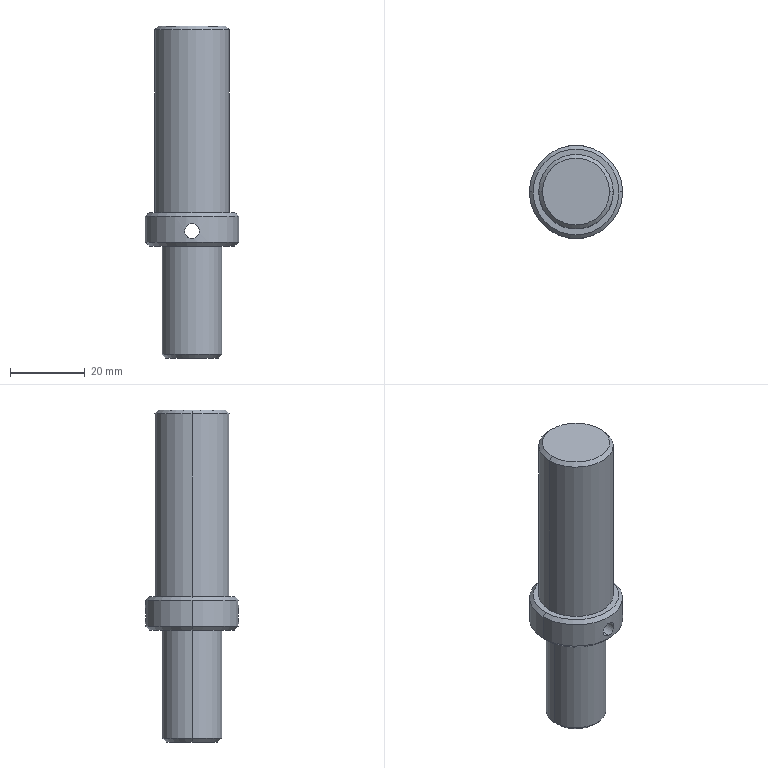Part | STEP file | Synchronous shaft 1 | 1 solid | 25 faces | box 25 x 25 x 89 mm | volume 25420 mm3 | cylinder 10 | cone 10 | plane 5 | commonest cylinder face diameters 4 x2 6 x2 16 x2 20 x2 25 x2
STEP:
#1=CARTESIAN_POINT('',(-10.,0.,88.));
#2=VERTEX_POINT('',#1);
#3=CARTESIAN_POINT('',(10.,0.,88.));
#4=VERTEX_POINT('',#3);
#5=CARTESIAN_POINT('',(0.,0.,88.));
#6=DIRECTION('',(0.,0.,-1.));
#7=DIRECTION('',(-1.,0.,0.));
#8=AXIS2_PLACEMENT_3D('',#5,#6,#7);
#9=CIRCLE('',#8,10.);
#10=EDGE_CURVE('',#2,#4,#9,.T.);
#11=ORIENTED_EDGE('',*,*,#10,.T.);
#12=CARTESIAN_POINT('',(10.,0.,39.));
#13=VERTEX_POINT('',#12);
#14=CARTESIAN_POINT('',(10.,0.,89.));
#15=DIRECTION('',(0.,0.,-1.));
#16=VECTOR('',#15,1000.);
#17=LINE('',#14,#16);
#18=EDGE_CURVE('',#4,#13,#17,.T.);
#19=ORIENTED_EDGE('',*,*,#18,.T.);
#20=CARTESIAN_POINT('',(-10.,0.,39.));
#21=VERTEX_POINT('',#20);
#22=CARTESIAN_POINT('',(0.,0.,39.));
#23=DIRECTION('',(0.,0.,1.));
#24=DIRECTION('',(-1.,0.,0.));
#25=AXIS2_PLACEMENT_3D('',#22,#23,#24);
#26=CIRCLE('',#25,10.);
#27=EDGE_CURVE('',#13,#21,#26,.T.);
#28=ORIENTED_EDGE('',*,*,#27,.T.);
#29=CARTESIAN_POINT('',(-10.,0.,89.));
#30=DIRECTION('',(0.,0.,-1.));
#31=VECTOR('',#30,1000.);
#32=LINE('',#29,#31);
#33=EDGE_CURVE('',#2,#21,#32,.T.);
#34=ORIENTED_EDGE('',*,*,#33,.F.);
#35=EDGE_LOOP('',(#11,#19,#28,#34));
#36=FACE_OUTER_BOUND('',#35,.T.);
#37=CARTESIAN_POINT('',(0.,0.,89.));
#38=DIRECTION('',(0.,0.,-1.));
#39=DIRECTION('',(-1.,0.,0.));
#40=AXIS2_PLACEMENT_3D('',#37,#38,#39);
#41=CYLINDRICAL_SURFACE('',#40,10.);
#42=ADVANCED_FACE('',(#36),#41,.T.);
#43=CARTESIAN_POINT('',(-9.,0.,89.));
#44=VERTEX_POINT('',#43);
#45=CARTESIAN_POINT('',(9.,0.,89.));
#46=VERTEX_POINT('',#45);
#47=CARTESIAN_POINT('',(0.,0.,89.));
#48=DIRECTION('',(0.,0.,-1.));
#49=DIRECTION('',(-1.,0.,0.));
#50=AXIS2_PLACEMENT_3D('',#47,#48,#49);
#51=CIRCLE('',#50,9.);
#52=EDGE_CURVE('',#44,#46,#51,.T.);
#53=ORIENTED_EDGE('',*,*,#52,.T.);
#54=CARTESIAN_POINT('',(10.,0.,88.));
#55=DIRECTION('',(0.7071,0.,-0.7071));
#56=VECTOR('',#55,1000.);
#57=LINE('',#54,#56);
#58=EDGE_CURVE('',#46,#4,#57,.T.);
#59=ORIENTED_EDGE('',*,*,#58,.T.);
#60=ORIENTED_EDGE('',*,*,#10,.F.);
#61=CARTESIAN_POINT('',(-10.,0.,88.));
#62=DIRECTION('',(-0.7071,0.,-0.7071));
#63=VECTOR('',#62,1000.);
#64=LINE('',#61,#63);
#65=EDGE_CURVE('',#44,#2,#64,.T.);
#66=ORIENTED_EDGE('',*,*,#65,.F.);
#67=EDGE_LOOP('',(#53,#59,#60,#66));
#68=FACE_OUTER_BOUND('',#67,.T.);
#69=CARTESIAN_POINT('',(0.,0.,88.));
#70=DIRECTION('',(0.,0.,-1.));
#71=DIRECTION('',(-1.,0.,0.));
#72=AXIS2_PLACEMENT_3D('',#69,#70,#71);
#73=CONICAL_SURFACE('',#72,10.,0.7854);
#74=ADVANCED_FACE('',(#68),#73,.T.);
#75=CARTESIAN_POINT('',(11.5,0.,39.));
#76=VERTEX_POINT('',#75);
#77=CARTESIAN_POINT('',(-11.5,0.,39.));
#78=VERTEX_POINT('',#77);
#79=CARTESIAN_POINT('',(0.,0.,39.));
#80=DIRECTION('',(0.,0.,1.));
#81=DIRECTION('',(-1.,0.,0.));
#82=AXIS2_PLACEMENT_3D('',#79,#80,#81);
#83=CIRCLE('',#82,11.5);
#84=EDGE_CURVE('',#76,#78,#83,.T.);
#85=ORIENTED_EDGE('',*,*,#84,.F.);
#86=CARTESIAN_POINT('',(12.5,0.,38.));
#87=VERTEX_POINT('',#86);
#88=CARTESIAN_POINT('',(12.5,0.,38.));
#89=DIRECTION('',(0.7071,0.,-0.7071));
#90=VECTOR('',#89,1000.);
#91=LINE('',#88,#90);
#92=EDGE_CURVE('',#76,#87,#91,.T.);
#93=ORIENTED_EDGE('',*,*,#92,.T.);
#94=CARTESIAN_POINT('',(-12.5,0.,38.));
#95=VERTEX_POINT('',#94);
#96=CARTESIAN_POINT('',(0.,0.,38.));
#97=DIRECTION('',(0.,0.,1.));
#98=DIRECTION('',(-1.,0.,0.));
#99=AXIS2_PLACEMENT_3D('',#96,#97,#98);
#100=CIRCLE('',#99,12.5);
#101=EDGE_CURVE('',#87,#95,#100,.T.);
#102=ORIENTED_EDGE('',*,*,#101,.T.);
#103=CARTESIAN_POINT('',(-12.5,0.,38.));
#104=DIRECTION('',(-0.7071,0.,-0.7071));
#105=VECTOR('',#104,1000.);
#106=LINE('',#103,#105);
#107=EDGE_CURVE('',#78,#95,#106,.T.);
#108=ORIENTED_EDGE('',*,*,#107,.F.);
#109=EDGE_LOOP('',(#85,#93,#102,#108));
#110=FACE_OUTER_BOUND('',#109,.T.);
#111=CARTESIAN_POINT('',(0.,0.,38.));
#112=DIRECTION('',(0.,0.,-1.));
#113=DIRECTION('',(-1.,0.,0.));
#114=AXIS2_PLACEMENT_3D('',#111,#112,#113);
#115=CONICAL_SURFACE('',#114,12.5,0.7854);
#116=ADVANCED_FACE('',(#110),#115,.T.);
#117=CARTESIAN_POINT('',(0.,12.5,36.));
#118=VERTEX_POINT('',#117);
#119=CARTESIAN_POINT('',(0.,12.5,32.));
#120=VERTEX_POINT('',#119);
#121=CARTESIAN_POINT('',(0.,12.5,36.));
#122=CARTESIAN_POINT('',(-0.1323,12.5,36.));
#123=CARTESIAN_POINT('',(-0.2624,12.498,35.987));
#124=CARTESIAN_POINT('',(-0.5183,12.49,35.936));
#125=CARTESIAN_POINT('',(-0.6454,12.484,35.898));
#126=CARTESIAN_POINT('',(-0.8875,12.469,35.797));
#127=CARTESIAN_POINT('',(-1.002,12.46,35.736));
#128=CARTESIAN_POINT('',(-1.219,12.441,35.591));
#129=CARTESIAN_POINT('',(-1.322,12.43,35.506));
#130=CARTESIAN_POINT('',(-1.598,12.399,35.23));
#131=CARTESIAN_POINT('',(-1.747,12.378,35.007));
#132=CARTESIAN_POINT('',(-1.947,12.348,34.526));
#133=CARTESIAN_POINT('',(-2.,12.339,34.263));
#134=CARTESIAN_POINT('',(-2.,12.339,33.871));
#135=CARTESIAN_POINT('',(-1.987,12.341,33.738));
#136=CARTESIAN_POINT('',(-1.936,12.349,33.481));
#137=CARTESIAN_POINT('',(-1.898,12.355,33.357));
#138=CARTESIAN_POINT('',(-1.798,12.37,33.114));
#139=CARTESIAN_POINT('',(-1.736,12.379,32.998));
#140=CARTESIAN_POINT('',(-1.591,12.399,32.781));
#141=CARTESIAN_POINT('',(-1.508,12.409,32.68));
#142=CARTESIAN_POINT('',(-1.322,12.43,32.493));
#143=CARTESIAN_POINT('',(-1.221,12.441,32.411));
#144=CARTESIAN_POINT('',(-1.005,12.46,32.266));
#145=CARTESIAN_POINT('',(-0.888,12.469,32.203));
#146=CARTESIAN_POINT('',(-0.6461,12.484,32.103));
#147=CARTESIAN_POINT('',(-0.5215,12.49,32.065));
#148=CARTESIAN_POINT('',(-0.2648,12.498,32.013));
#149=CARTESIAN_POINT('',(-0.1323,12.5,32.));
#150=CARTESIAN_POINT('',(0.,12.5,32.));
#151=B_SPLINE_CURVE_WITH_KNOTS('',3,(#121,#122,#123,#124,#125,#126,#127,#128,#129,#130,#131,#132,#133,#134,#135,#136,#137,#138,#139,#140,#141,#142,#143,#144,#145,#146,#147,#148,#149,#150),.UNSPECIFIED.,.F.,.F.,(4,2,2,2,2,2,2,2,2,2,2,2,2,2,4),(0.006261,0.006653,0.007044,0.007435,0.007827,0.008609,0.009392,0.009783,0.01017,0.01057,0.01096,0.01135,0.01174,0.01213,0.01252),.UNSPECIFIED.);
#152=EDGE_CURVE('',#118,#120,#151,.T.);
#153=ORIENTED_EDGE('',*,*,#152,.T.);
#154=CARTESIAN_POINT('',(0.,12.5,32.));
#155=CARTESIAN_POINT('',(0.1323,12.5,32.));
#156=CARTESIAN_POINT('',(0.2624,12.498,32.013));
#157=CARTESIAN_POINT('',(0.5183,12.49,32.064));
#158=CARTESIAN_POINT('',(0.6454,12.484,32.102));
#159=CARTESIAN_POINT('',(0.8875,12.469,32.203));
#160=CARTESIAN_POINT('',(1.002,12.46,32.264));
#161=CARTESIAN_POINT('',(1.219,12.441,32.409));
#162=CARTESIAN_POINT('',(1.322,12.43,32.494));
#163=CARTESIAN_POINT('',(1.598,12.399,32.77));
#164=CARTESIAN_POINT('',(1.747,12.378,32.993));
#165=CARTESIAN_POINT('',(1.947,12.348,33.474));
#166=CARTESIAN_POINT('',(2.,12.339,33.737));
#167=CARTESIAN_POINT('',(2.,12.339,34.129));
#168=CARTESIAN_POINT('',(1.987,12.341,34.262));
#169=CARTESIAN_POINT('',(1.936,12.349,34.519));
#170=CARTESIAN_POINT('',(1.898,12.355,34.643));
#171=CARTESIAN_POINT('',(1.798,12.37,34.886));
#172=CARTESIAN_POINT('',(1.736,12.379,35.002));
#173=CARTESIAN_POINT('',(1.591,12.399,35.219));
#174=CARTESIAN_POINT('',(1.508,12.409,35.32));
#175=CARTESIAN_POINT('',(1.322,12.43,35.507));
#176=CARTESIAN_POINT('',(1.221,12.441,35.589));
#177=CARTESIAN_POINT('',(1.005,12.46,35.734));
#178=CARTESIAN_POINT('',(0.888,12.469,35.797));
#179=CARTESIAN_POINT('',(0.6461,12.484,35.897));
#180=CARTESIAN_POINT('',(0.5215,12.49,35.935));
#181=CARTESIAN_POINT('',(0.2648,12.498,35.987));
#182=CARTESIAN_POINT('',(0.1323,12.5,36.));
#183=CARTESIAN_POINT('',(0.,12.5,36.));
#184=B_SPLINE_CURVE_WITH_KNOTS('',3,(#154,#155,#156,#157,#158,#159,#160,#161,#162,#163,#164,#165,#166,#167,#168,#169,#170,#171,#172,#173,#174,#175,#176,#177,#178,#179,#180,#181,#182,#183),.UNSPECIFIED.,.F.,.F.,(4,2,2,2,2,2,2,2,2,2,2,2,2,2,4),(0.,0.0003913,0.0007827,0.001174,0.001565,0.002348,0.003131,0.003522,0.003913,0.004305,0.004696,0.005087,0.005479,0.00587,0.006261),.UNSPECIFIED.);
#185=EDGE_CURVE('',#120,#118,#184,.T.);
#186=ORIENTED_EDGE('',*,*,#185,.T.);
#187=EDGE_LOOP('',(#153,#186));
#188=FACE_BOUND('',#187,.T.);
#189=ORIENTED_EDGE('',*,*,#101,.F.);
#190=CARTESIAN_POINT('',(12.5,0.,31.));
#191=VERTEX_POINT('',#190);
#192=CARTESIAN_POINT('',(12.5,0.,39.));
#193=DIRECTION('',(0.,0.,-1.));
#194=VECTOR('',#193,1000.);
#195=LINE('',#192,#194);
#196=EDGE_CURVE('',#87,#191,#195,.T.);
#197=ORIENTED_EDGE('',*,*,#196,.T.);
#198=CARTESIAN_POINT('',(-12.5,0.,31.));
#199=VERTEX_POINT('',#198);
#200=CARTESIAN_POINT('',(0.,0.,31.));
#201=DIRECTION('',(0.,0.,1.));
#202=DIRECTION('',(-1.,0.,0.));
#203=AXIS2_PLACEMENT_3D('',#200,#201,#202);
#204=CIRCLE('',#203,12.5);
#205=EDGE_CURVE('',#191,#199,#204,.T.);
#206=ORIENTED_EDGE('',*,*,#205,.T.);
#207=CARTESIAN_POINT('',(-12.5,0.,39.));
#208=DIRECTION('',(0.,0.,-1.));
#209=VECTOR('',#208,1000.);
#210=LINE('',#207,#209);
#211=EDGE_CURVE('',#95,#199,#210,.T.);
#212=ORIENTED_EDGE('',*,*,#211,.F.);
#213=EDGE_LOOP('',(#189,#197,#206,#212));
#214=FACE_OUTER_BOUND('',#213,.T.);
#215=CARTESIAN_POINT('',(0.,0.,39.));
#216=DIRECTION('',(0.,0.,-1.));
#217=DIRECTION('',(-1.,0.,0.));
#218=AXIS2_PLACEMENT_3D('',#215,#216,#217);
#219=CYLINDRICAL_SURFACE('',#218,12.5);
#220=ADVANCED_FACE('',(#188,#214),#219,.T.);
#221=CARTESIAN_POINT('',(11.5,0.,30.));
#222=VERTEX_POINT('',#221);
#223=CARTESIAN_POINT('',(-11.5,0.,30.));
#224=VERTEX_POINT('',#223);
#225=CARTESIAN_POINT('',(0.,0.,30.));
#226=DIRECTION('',(0.,0.,1.));
#227=DIRECTION('',(1.,0.,0.));
#228=AXIS2_PLACEMENT_3D('',#225,#226,#227);
#229=CIRCLE('',#228,11.5);
#230=EDGE_CURVE('',#222,#224,#229,.T.);
#231=ORIENTED_EDGE('',*,*,#230,.T.);
#232=CARTESIAN_POINT('',(-12.5,0.,31.));
#233=DIRECTION('',(-0.7071,0.,0.7071));
#234=VECTOR('',#233,1000.);
#235=LINE('',#232,#234);
#236=EDGE_CURVE('',#224,#199,#235,.T.);
#237=ORIENTED_EDGE('',*,*,#236,.T.);
#238=ORIENTED_EDGE('',*,*,#205,.F.);
#239=CARTESIAN_POINT('',(12.5,0.,31.));
#240=DIRECTION('',(0.7071,0.,0.7071));
#241=VECTOR('',#240,1000.);
#242=LINE('',#239,#241);
#243=EDGE_CURVE('',#222,#191,#242,.T.);
#244=ORIENTED_EDGE('',*,*,#243,.F.);
#245=EDGE_LOOP('',(#231,#237,#238,#244));
#246=FACE_OUTER_BOUND('',#245,.T.);
#247=CARTESIAN_POINT('',(0.,0.,31.));
#248=DIRECTION('',(0.,0.,1.));
#249=DIRECTION('',(1.,0.,0.));
#250=AXIS2_PLACEMENT_3D('',#247,#248,#249);
#251=CONICAL_SURFACE('',#250,12.5,0.7854);
#252=ADVANCED_FACE('',(#246),#251,.T.);
#253=CARTESIAN_POINT('',(0.,-12.5,32.));
#254=VERTEX_POINT('',#253);
#255=CARTESIAN_POINT('',(0.,-12.5,36.));
#256=VERTEX_POINT('',#255);
#257=CARTESIAN_POINT('',(0.,-12.5,32.));
#258=CARTESIAN_POINT('',(-0.1323,-12.5,32.));
#259=CARTESIAN_POINT('',(-0.2624,-12.498,32.013));
#260=CARTESIAN_POINT('',(-0.5183,-12.49,32.064));
#261=CARTESIAN_POINT('',(-0.6454,-12.484,32.102));
#262=CARTESIAN_POINT('',(-0.8875,-12.469,32.203));
#263=CARTESIAN_POINT('',(-1.002,-12.46,32.264));
#264=CARTESIAN_POINT('',(-1.219,-12.441,32.409));
#265=CARTESIAN_POINT('',(-1.322,-12.43,32.494));
#266=CARTESIAN_POINT('',(-1.598,-12.399,32.77));
#267=CARTESIAN_POINT('',(-1.747,-12.378,32.993));
#268=CARTESIAN_POINT('',(-1.947,-12.348,33.474));
#269=CARTESIAN_POINT('',(-2.,-12.339,33.737));
#270=CARTESIAN_POINT('',(-2.,-12.339,34.129));
#271=CARTESIAN_POINT('',(-1.987,-12.341,34.262));
#272=CARTESIAN_POINT('',(-1.936,-12.349,34.519));
#273=CARTESIAN_POINT('',(-1.898,-12.355,34.643));
#274=CARTESIAN_POINT('',(-1.798,-12.37,34.886));
#275=CARTESIAN_POINT('',(-1.736,-12.379,35.002));
#276=CARTESIAN_POINT('',(-1.591,-12.399,35.219));
#277=CARTESIAN_POINT('',(-1.508,-12.409,35.32));
#278=CARTESIAN_POINT('',(-1.322,-12.43,35.507));
#279=CARTESIAN_POINT('',(-1.221,-12.441,35.589));
#280=CARTESIAN_POINT('',(-1.005,-12.46,35.734));
#281=CARTESIAN_POINT('',(-0.888,-12.469,35.797));
#282=CARTESIAN_POINT('',(-0.6461,-12.484,35.897));
#283=CARTESIAN_POINT('',(-0.5215,-12.49,35.935));
#284=CARTESIAN_POINT('',(-0.2648,-12.498,35.987));
#285=CARTESIAN_POINT('',(-0.1323,-12.5,36.));
#286=CARTESIAN_POINT('',(0.,-12.5,36.));
#287=B_SPLINE_CURVE_WITH_KNOTS('',3,(#257,#258,#259,#260,#261,#262,#263,#264,#265,#266,#267,#268,#269,#270,#271,#272,#273,#274,#275,#276,#277,#278,#279,#280,#281,#282,#283,#284,#285,#286),.UNSPECIFIED.,.F.,.F.,(4,2,2,2,2,2,2,2,2,2,2,2,2,2,4),(0.,0.0003913,0.0007827,0.001174,0.001565,0.002348,0.003131,0.003522,0.003913,0.004305,0.004696,0.005087,0.005479,0.00587,0.006261),.UNSPECIFIED.);
#288=EDGE_CURVE('',#254,#256,#287,.T.);
#289=ORIENTED_EDGE('',*,*,#288,.F.);
#290=CARTESIAN_POINT('',(0.,-15.,32.));
#291=DIRECTION('',(0.,1.,0.));
#292=VECTOR('',#291,1000.);
#293=LINE('',#290,#292);
#294=EDGE_CURVE('',#254,#120,#293,.T.);
#295=ORIENTED_EDGE('',*,*,#294,.T.);
#296=ORIENTED_EDGE('',*,*,#152,.F.);
#297=CARTESIAN_POINT('',(0.,-15.,36.));
#298=DIRECTION('',(0.,1.,0.));
#299=VECTOR('',#298,1000.);
#300=LINE('',#297,#299);
#301=EDGE_CURVE('',#256,#118,#300,.T.);
#302=ORIENTED_EDGE('',*,*,#301,.F.);
#303=EDGE_LOOP('',(#289,#295,#296,#302));
#304=FACE_OUTER_BOUND('',#303,.T.);
#305=CARTESIAN_POINT('',(0.,-15.,34.));
#306=DIRECTION('',(0.,1.,0.));
#307=DIRECTION('',(0.,0.,1.));
#308=AXIS2_PLACEMENT_3D('',#305,#306,#307);
#309=CYLINDRICAL_SURFACE('',#308,2.);
#310=ADVANCED_FACE('',(#304),#309,.F.);
#311=CARTESIAN_POINT('',(-8.,0.,30.));
#312=VERTEX_POINT('',#311);
#313=CARTESIAN_POINT('',(8.,0.,30.));
#314=VERTEX_POINT('',#313);
#315=CARTESIAN_POINT('',(0.,0.,30.));
#316=DIRECTION('',(0.,0.,-1.));
#317=DIRECTION('',(-1.,0.,0.));
#318=AXIS2_PLACEMENT_3D('',#315,#316,#317);
#319=CIRCLE('',#318,8.);
#320=EDGE_CURVE('',#312,#314,#319,.T.);
#321=ORIENTED_EDGE('',*,*,#320,.T.);
#322=CARTESIAN_POINT('',(8.,0.,1.));
#323=VERTEX_POINT('',#322);
#324=CARTESIAN_POINT('',(8.,0.,30.));
#325=DIRECTION('',(0.,0.,-1.));
#326=VECTOR('',#325,1000.);
#327=LINE('',#324,#326);
#328=EDGE_CURVE('',#314,#323,#327,.T.);
#329=ORIENTED_EDGE('',*,*,#328,.T.);
#330=CARTESIAN_POINT('',(-8.,0.,1.));
#331=VERTEX_POINT('',#330);
#332=CARTESIAN_POINT('',(0.,0.,1.));
#333=DIRECTION('',(0.,0.,1.));
#334=DIRECTION('',(-1.,0.,0.));
#335=AXIS2_PLACEMENT_3D('',#332,#333,#334);
#336=CIRCLE('',#335,8.);
#337=EDGE_CURVE('',#323,#331,#336,.T.);
#338=ORIENTED_EDGE('',*,*,#337,.T.);
#339=CARTESIAN_POINT('',(-8.,0.,30.));
#340=DIRECTION('',(0.,0.,-1.));
#341=VECTOR('',#340,1000.);
#342=LINE('',#339,#341);
#343=EDGE_CURVE('',#312,#331,#342,.T.);
#344=ORIENTED_EDGE('',*,*,#343,.F.);
#345=EDGE_LOOP('',(#321,#329,#338,#344));
#346=FACE_OUTER_BOUND('',#345,.T.);
#347=CARTESIAN_POINT('',(0.,0.,30.));
#348=DIRECTION('',(0.,0.,-1.));
#349=DIRECTION('',(-1.,0.,0.));
#350=AXIS2_PLACEMENT_3D('',#347,#348,#349);
#351=CYLINDRICAL_SURFACE('',#350,8.);
#352=ADVANCED_FACE('',(#346),#351,.T.);
#353=CARTESIAN_POINT('',(7.,0.,0.));
#354=VERTEX_POINT('',#353);
#355=CARTESIAN_POINT('',(-7.,0.,0.));
#356=VERTEX_POINT('',#355);
#357=CARTESIAN_POINT('',(0.,0.,0.));
#358=DIRECTION('',(0.,0.,1.));
#359=DIRECTION('',(1.,0.,0.));
#360=AXIS2_PLACEMENT_3D('',#357,#358,#359);
#361=CIRCLE('',#360,7.);
#362=EDGE_CURVE('',#354,#356,#361,.T.);
#363=ORIENTED_EDGE('',*,*,#362,.T.);
#364=CARTESIAN_POINT('',(-8.,0.,1.));
#365=DIRECTION('',(-0.7071,0.,0.7071));
#366=VECTOR('',#365,1000.);
#367=LINE('',#364,#366);
#368=EDGE_CURVE('',#356,#331,#367,.T.);
#369=ORIENTED_EDGE('',*,*,#368,.T.);
#370=ORIENTED_EDGE('',*,*,#337,.F.);
#371=CARTESIAN_POINT('',(8.,0.,1.));
#372=DIRECTION('',(0.7071,0.,0.7071));
#373=VECTOR('',#372,1000.);
#374=LINE('',#371,#373);
#375=EDGE_CURVE('',#354,#323,#374,.T.);
#376=ORIENTED_EDGE('',*,*,#375,.F.);
#377=EDGE_LOOP('',(#363,#369,#370,#376));
#378=FACE_OUTER_BOUND('',#377,.T.);
#379=CARTESIAN_POINT('',(0.,0.,1.));
#380=DIRECTION('',(0.,0.,1.));
#381=DIRECTION('',(1.,0.,0.));
#382=AXIS2_PLACEMENT_3D('',#379,#380,#381);
#383=CONICAL_SURFACE('',#382,8.,0.7854);
#384=ADVANCED_FACE('',(#378),#383,.T.);
#385=CARTESIAN_POINT('',(3.,0.,1.));
#386=VERTEX_POINT('',#385);
#387=CARTESIAN_POINT('',(-3.,0.,1.));
#388=VERTEX_POINT('',#387);
#389=CARTESIAN_POINT('',(0.,0.,1.));
#390=DIRECTION('',(0.,0.,-1.));
#391=DIRECTION('',(-1.,0.,0.));
#392=AXIS2_PLACEMENT_3D('',#389,#390,#391);
#393=CIRCLE('',#392,3.);
#394=EDGE_CURVE('',#386,#388,#393,.T.);
#395=ORIENTED_EDGE('',*,*,#394,.F.);
#396=CARTESIAN_POINT('',(4.,0.,0.));
#397=VERTEX_POINT('',#396);
#398=CARTESIAN_POINT('',(4.,0.,0.));
#399=DIRECTION('',(0.7071,0.,-0.7071));
#400=VECTOR('',#399,1000.);
#401=LINE('',#398,#400);
#402=EDGE_CURVE('',#386,#397,#401,.T.);
#403=ORIENTED_EDGE('',*,*,#402,.T.);
#404=CARTESIAN_POINT('',(-4.,0.,0.));
#405=VERTEX_POINT('',#404);
#406=CARTESIAN_POINT('',(0.,0.,0.));
#407=DIRECTION('',(0.,0.,-1.));
#408=DIRECTION('',(-1.,0.,0.));
#409=AXIS2_PLACEMENT_3D('',#406,#407,#408);
#410=CIRCLE('',#409,4.);
#411=EDGE_CURVE('',#397,#405,#410,.T.);
#412=ORIENTED_EDGE('',*,*,#411,.T.);
#413=CARTESIAN_POINT('',(-4.,0.,0.));
#414=DIRECTION('',(-0.7071,0.,-0.7071));
#415=VECTOR('',#414,1000.);
#416=LINE('',#413,#415);
#417=EDGE_CURVE('',#388,#405,#416,.T.);
#418=ORIENTED_EDGE('',*,*,#417,.F.);
#419=EDGE_LOOP('',(#395,#403,#412,#418));
#420=FACE_OUTER_BOUND('',#419,.T.);
#421=CARTESIAN_POINT('',(0.,0.,0.));
#422=DIRECTION('',(0.,0.,-1.));
#423=DIRECTION('',(-1.,0.,0.));
#424=AXIS2_PLACEMENT_3D('',#421,#422,#423);
#425=CONICAL_SURFACE('',#424,4.,0.7854);
#426=ADVANCED_FACE('',(#420),#425,.F.);
#427=CARTESIAN_POINT('',(3.,0.,10.));
#428=VERTEX_POINT('',#427);
#429=CARTESIAN_POINT('',(-3.,0.,10.));
#430=VERTEX_POINT('',#429);
#431=CARTESIAN_POINT('',(0.,0.,10.));
#432=DIRECTION('',(0.,0.,-1.));
#433=DIRECTION('',(-1.,0.,0.));
#434=AXIS2_PLACEMENT_3D('',#431,#432,#433);
#435=CIRCLE('',#434,3.);
#436=EDGE_CURVE('',#428,#430,#435,.T.);
#437=ORIENTED_EDGE('',*,*,#436,.F.);
#438=CARTESIAN_POINT('',(3.,0.,10.));
#439=DIRECTION('',(0.,0.,-1.));
#440=VECTOR('',#439,1000.);
#441=LINE('',#438,#440);
#442=EDGE_CURVE('',#428,#386,#441,.T.);
#443=ORIENTED_EDGE('',*,*,#442,.T.);
#444=ORIENTED_EDGE('',*,*,#394,.T.);
#445=CARTESIAN_POINT('',(-3.,0.,10.));
#446=DIRECTION('',(0.,0.,-1.));
#447=VECTOR('',#446,1000.);
#448=LINE('',#445,#447);
#449=EDGE_CURVE('',#430,#388,#448,.T.);
#450=ORIENTED_EDGE('',*,*,#449,.F.);
#451=EDGE_LOOP('',(#437,#443,#444,#450));
#452=FACE_OUTER_BOUND('',#451,.T.);
#453=CARTESIAN_POINT('',(0.,0.,10.));
#454=DIRECTION('',(0.,0.,-1.));
#455=DIRECTION('',(-1.,0.,0.));
#456=AXIS2_PLACEMENT_3D('',#453,#454,#455);
#457=CYLINDRICAL_SURFACE('',#456,3.);
#458=ADVANCED_FACE('',(#452),#457,.F.);
#459=ORIENTED_EDGE('',*,*,#18,.F.);
#460=CARTESIAN_POINT('',(0.,0.,88.));
#461=DIRECTION('',(0.,0.,-1.));
#462=DIRECTION('',(-1.,0.,0.));
#463=AXIS2_PLACEMENT_3D('',#460,#461,#462);
#464=CIRCLE('',#463,10.);
#465=EDGE_CURVE('',#4,#2,#464,.T.);
#466=ORIENTED_EDGE('',*,*,#465,.T.);
#467=ORIENTED_EDGE('',*,*,#33,.T.);
#468=CARTESIAN_POINT('',(0.,0.,39.));
#469=DIRECTION('',(0.,0.,1.));
#470=DIRECTION('',(-1.,0.,0.));
#471=AXIS2_PLACEMENT_3D('',#468,#469,#470);
#472=CIRCLE('',#471,10.);
#473=EDGE_CURVE('',#21,#13,#472,.T.);
#474=ORIENTED_EDGE('',*,*,#473,.T.);
#475=EDGE_LOOP('',(#459,#466,#467,#474));
#476=FACE_OUTER_BOUND('',#475,.T.);
#477=CARTESIAN_POINT('',(0.,0.,89.));
#478=DIRECTION('',(0.,0.,-1.));
#479=DIRECTION('',(-1.,0.,0.));
#480=AXIS2_PLACEMENT_3D('',#477,#478,#479);
#481=CYLINDRICAL_SURFACE('',#480,10.);
#482=ADVANCED_FACE('',(#476),#481,.T.);
#483=ORIENTED_EDGE('',*,*,#473,.F.);
#484=ORIENTED_EDGE('',*,*,#27,.F.);
#485=EDGE_LOOP('',(#483,#484));
#486=FACE_BOUND('',#485,.T.);
#487=CARTESIAN_POINT('',(0.,0.,39.));
#488=DIRECTION('',(0.,0.,1.));
#489=DIRECTION('',(-1.,0.,0.));
#490=AXIS2_PLACEMENT_3D('',#487,#488,#489);
#491=CIRCLE('',#490,11.5);
#492=EDGE_CURVE('',#78,#76,#491,.T.);
#493=ORIENTED_EDGE('',*,*,#492,.T.);
#494=ORIENTED_EDGE('',*,*,#84,.T.);
#495=EDGE_LOOP('',(#493,#494));
#496=FACE_OUTER_BOUND('',#495,.T.);
#497=CARTESIAN_POINT('',(0.,0.,39.));
#498=DIRECTION('',(0.,0.,1.));
#499=DIRECTION('',(1.,0.,0.));
#500=AXIS2_PLACEMENT_3D('',#497,#498,#499);
#501=PLANE('',#500);
#502=ADVANCED_FACE('',(#486,#496),#501,.T.);
#503=ORIENTED_EDGE('',*,*,#58,.F.);
#504=CARTESIAN_POINT('',(0.,0.,89.));
#505=DIRECTION('',(0.,0.,-1.));
#506=DIRECTION('',(-1.,0.,0.));
#507=AXIS2_PLACEMENT_3D('',#504,#505,#506);
#508=CIRCLE('',#507,9.);
#509=EDGE_CURVE('',#46,#44,#508,.T.);
#510=ORIENTED_EDGE('',*,*,#509,.T.);
#511=ORIENTED_EDGE('',*,*,#65,.T.);
#512=ORIENTED_EDGE('',*,*,#465,.F.);
#513=EDGE_LOOP('',(#503,#510,#511,#512));
#514=FACE_OUTER_BOUND('',#513,.T.);
#515=CARTESIAN_POINT('',(0.,0.,88.));
#516=DIRECTION('',(0.,0.,-1.));
#517=DIRECTION('',(-1.,0.,0.));
#518=AXIS2_PLACEMENT_3D('',#515,#516,#517);
#519=CONICAL_SURFACE('',#518,10.,0.7854);
#520=ADVANCED_FACE('',(#514),#519,.T.);
#521=ORIENTED_EDGE('',*,*,#92,.F.);
#522=ORIENTED_EDGE('',*,*,#492,.F.);
#523=ORIENTED_EDGE('',*,*,#107,.T.);
#524=CARTESIAN_POINT('',(0.,0.,38.));
#525=DIRECTION('',(0.,0.,1.));
#526=DIRECTION('',(-1.,0.,0.));
#527=AXIS2_PLACEMENT_3D('',#524,#525,#526);
#528=CIRCLE('',#527,12.5);
#529=EDGE_CURVE('',#95,#87,#528,.T.);
#530=ORIENTED_EDGE('',*,*,#529,.T.);
#531=EDGE_LOOP('',(#521,#522,#523,#530));
#532=FACE_OUTER_BOUND('',#531,.T.);
#533=CARTESIAN_POINT('',(0.,0.,38.));
#534=DIRECTION('',(0.,0.,-1.));
#535=DIRECTION('',(-1.,0.,0.));
#536=AXIS2_PLACEMENT_3D('',#533,#534,#535);
#537=CONICAL_SURFACE('',#536,12.5,0.7854);
#538=ADVANCED_FACE('',(#532),#537,.T.);
#539=ORIENTED_EDGE('',*,*,#52,.F.);
#540=ORIENTED_EDGE('',*,*,#509,.F.);
#541=EDGE_LOOP('',(#539,#540));
#542=FACE_OUTER_BOUND('',#541,.T.);
#543=CARTESIAN_POINT('',(0.,0.,89.));
#544=DIRECTION('',(0.,0.,1.));
#545=DIRECTION('',(1.,0.,0.));
#546=AXIS2_PLACEMENT_3D('',#543,#544,#545);
#547=PLANE('',#546);
#548=ADVANCED_FACE('',(#542),#547,.T.);
#549=ORIENTED_EDGE('',*,*,#196,.F.);
#550=ORIENTED_EDGE('',*,*,#529,.F.);
#551=ORIENTED_EDGE('',*,*,#211,.T.);
#552=CARTESIAN_POINT('',(0.,0.,31.));
#553=DIRECTION('',(0.,0.,1.));
#554=DIRECTION('',(-1.,0.,0.));
#555=AXIS2_PLACEMENT_3D('',#552,#553,#554);
#556=CIRCLE('',#555,12.5);
#557=EDGE_CURVE('',#199,#191,#556,.T.);
#558=ORIENTED_EDGE('',*,*,#557,.T.);
#559=EDGE_LOOP('',(#549,#550,#551,#558));
#560=FACE_OUTER_BOUND('',#559,.T.);
#561=CARTESIAN_POINT('',(0.,-12.5,36.));
#562=CARTESIAN_POINT('',(0.1323,-12.5,36.));
#563=CARTESIAN_POINT('',(0.2624,-12.498,35.987));
#564=CARTESIAN_POINT('',(0.5183,-12.49,35.936));
#565=CARTESIAN_POINT('',(0.6454,-12.484,35.898));
#566=CARTESIAN_POINT('',(0.8875,-12.469,35.797));
#567=CARTESIAN_POINT('',(1.002,-12.46,35.736));
#568=CARTESIAN_POINT('',(1.219,-12.441,35.591));
#569=CARTESIAN_POINT('',(1.322,-12.43,35.506));
#570=CARTESIAN_POINT('',(1.598,-12.399,35.23));
#571=CARTESIAN_POINT('',(1.747,-12.378,35.007));
#572=CARTESIAN_POINT('',(1.947,-12.348,34.526));
#573=CARTESIAN_POINT('',(2.,-12.339,34.263));
#574=CARTESIAN_POINT('',(2.,-12.339,33.871));
#575=CARTESIAN_POINT('',(1.987,-12.341,33.738));
#576=CARTESIAN_POINT('',(1.936,-12.349,33.481));
#577=CARTESIAN_POINT('',(1.898,-12.355,33.357));
#578=CARTESIAN_POINT('',(1.798,-12.37,33.114));
#579=CARTESIAN_POINT('',(1.736,-12.379,32.998));
#580=CARTESIAN_POINT('',(1.591,-12.399,32.781));
#581=CARTESIAN_POINT('',(1.508,-12.409,32.68));
#582=CARTESIAN_POINT('',(1.322,-12.43,32.493));
#583=CARTESIAN_POINT('',(1.221,-12.441,32.411));
#584=CARTESIAN_POINT('',(1.005,-12.46,32.266));
#585=CARTESIAN_POINT('',(0.888,-12.469,32.203));
#586=CARTESIAN_POINT('',(0.6461,-12.484,32.103));
#587=CARTESIAN_POINT('',(0.5215,-12.49,32.065));
#588=CARTESIAN_POINT('',(0.2648,-12.498,32.013));
#589=CARTESIAN_POINT('',(0.1323,-12.5,32.));
#590=CARTESIAN_POINT('',(0.,-12.5,32.));
#591=B_SPLINE_CURVE_WITH_KNOTS('',3,(#561,#562,#563,#564,#565,#566,#567,#568,#569,#570,#571,#572,#573,#574,#575,#576,#577,#578,#579,#580,#581,#582,#583,#584,#585,#586,#587,#588,#589,#590),.UNSPECIFIED.,.F.,.F.,(4,2,2,2,2,2,2,2,2,2,2,2,2,2,4),(0.006261,0.006653,0.007044,0.007435,0.007827,0.008609,0.009392,0.009783,0.01017,0.01057,0.01096,0.01135,0.01174,0.01213,0.01252),.UNSPECIFIED.);
#592=EDGE_CURVE('',#256,#254,#591,.T.);
#593=ORIENTED_EDGE('',*,*,#592,.T.);
#594=ORIENTED_EDGE('',*,*,#288,.T.);
#595=EDGE_LOOP('',(#593,#594));
#596=FACE_BOUND('',#595,.T.);
#597=CARTESIAN_POINT('',(0.,0.,39.));
#598=DIRECTION('',(0.,0.,-1.));
#599=DIRECTION('',(-1.,0.,0.));
#600=AXIS2_PLACEMENT_3D('',#597,#598,#599);
#601=CYLINDRICAL_SURFACE('',#600,12.5);
#602=ADVANCED_FACE('',(#560,#596),#601,.T.);
#603=ORIENTED_EDGE('',*,*,#236,.F.);
#604=CARTESIAN_POINT('',(0.,0.,30.));
#605=DIRECTION('',(0.,0.,1.));
#606=DIRECTION('',(1.,0.,0.));
#607=AXIS2_PLACEMENT_3D('',#604,#605,#606);
#608=CIRCLE('',#607,11.5);
#609=EDGE_CURVE('',#224,#222,#608,.T.);
#610=ORIENTED_EDGE('',*,*,#609,.T.);
#611=ORIENTED_EDGE('',*,*,#243,.T.);
#612=ORIENTED_EDGE('',*,*,#557,.F.);
#613=EDGE_LOOP('',(#603,#610,#611,#612));
#614=FACE_OUTER_BOUND('',#613,.T.);
#615=CARTESIAN_POINT('',(0.,0.,31.));
#616=DIRECTION('',(0.,0.,1.));
#617=DIRECTION('',(1.,0.,0.));
#618=AXIS2_PLACEMENT_3D('',#615,#616,#617);
#619=CONICAL_SURFACE('',#618,12.5,0.7854);
#620=ADVANCED_FACE('',(#614),#619,.T.);
#621=ORIENTED_EDGE('',*,*,#294,.F.);
#622=ORIENTED_EDGE('',*,*,#592,.F.);
#623=ORIENTED_EDGE('',*,*,#301,.T.);
#624=ORIENTED_EDGE('',*,*,#185,.F.);
#625=EDGE_LOOP('',(#621,#622,#623,#624));
#626=FACE_OUTER_BOUND('',#625,.T.);
#627=CARTESIAN_POINT('',(0.,-15.,34.));
#628=DIRECTION('',(0.,1.,0.));
#629=DIRECTION('',(0.,0.,1.));
#630=AXIS2_PLACEMENT_3D('',#627,#628,#629);
#631=CYLINDRICAL_SURFACE('',#630,2.);
#632=ADVANCED_FACE('',(#626),#631,.F.);
#633=ORIENTED_EDGE('',*,*,#320,.F.);
#634=CARTESIAN_POINT('',(0.,0.,30.));
#635=DIRECTION('',(0.,0.,-1.));
#636=DIRECTION('',(-1.,0.,0.));
#637=AXIS2_PLACEMENT_3D('',#634,#635,#636);
#638=CIRCLE('',#637,8.);
#639=EDGE_CURVE('',#314,#312,#638,.T.);
#640=ORIENTED_EDGE('',*,*,#639,.F.);
#641=EDGE_LOOP('',(#633,#640));
#642=FACE_BOUND('',#641,.T.);
#643=ORIENTED_EDGE('',*,*,#230,.F.);
#644=ORIENTED_EDGE('',*,*,#609,.F.);
#645=EDGE_LOOP('',(#643,#644));
#646=FACE_OUTER_BOUND('',#645,.T.);
#647=CARTESIAN_POINT('',(0.,0.,30.));
#648=DIRECTION('',(0.,0.,1.));
#649=DIRECTION('',(1.,0.,0.));
#650=AXIS2_PLACEMENT_3D('',#647,#648,#649);
#651=PLANE('',#650);
#652=ADVANCED_FACE('',(#642,#646),#651,.F.);
#653=ORIENTED_EDGE('',*,*,#328,.F.);
#654=ORIENTED_EDGE('',*,*,#639,.T.);
#655=ORIENTED_EDGE('',*,*,#343,.T.);
#656=CARTESIAN_POINT('',(0.,0.,1.));
#657=DIRECTION('',(0.,0.,1.));
#658=DIRECTION('',(-1.,0.,0.));
#659=AXIS2_PLACEMENT_3D('',#656,#657,#658);
#660=CIRCLE('',#659,8.);
#661=EDGE_CURVE('',#331,#323,#660,.T.);
#662=ORIENTED_EDGE('',*,*,#661,.T.);
#663=EDGE_LOOP('',(#653,#654,#655,#662));
#664=FACE_OUTER_BOUND('',#663,.T.);
#665=CARTESIAN_POINT('',(0.,0.,30.));
#666=DIRECTION('',(0.,0.,-1.));
#667=DIRECTION('',(-1.,0.,0.));
#668=AXIS2_PLACEMENT_3D('',#665,#666,#667);
#669=CYLINDRICAL_SURFACE('',#668,8.);
#670=ADVANCED_FACE('',(#664),#669,.T.);
#671=ORIENTED_EDGE('',*,*,#368,.F.);
#672=CARTESIAN_POINT('',(0.,0.,0.));
#673=DIRECTION('',(0.,0.,1.));
#674=DIRECTION('',(1.,0.,0.));
#675=AXIS2_PLACEMENT_3D('',#672,#673,#674);
#676=CIRCLE('',#675,7.);
#677=EDGE_CURVE('',#356,#354,#676,.T.);
#678=ORIENTED_EDGE('',*,*,#677,.T.);
#679=ORIENTED_EDGE('',*,*,#375,.T.);
#680=ORIENTED_EDGE('',*,*,#661,.F.);
#681=EDGE_LOOP('',(#671,#678,#679,#680));
#682=FACE_OUTER_BOUND('',#681,.T.);
#683=CARTESIAN_POINT('',(0.,0.,1.));
#684=DIRECTION('',(0.,0.,1.));
#685=DIRECTION('',(1.,0.,0.));
#686=AXIS2_PLACEMENT_3D('',#683,#684,#685);
#687=CONICAL_SURFACE('',#686,8.,0.7854);
#688=ADVANCED_FACE('',(#682),#687,.T.);
#689=ORIENTED_EDGE('',*,*,#362,.F.);
#690=ORIENTED_EDGE('',*,*,#677,.F.);
#691=EDGE_LOOP('',(#689,#690));
#692=FACE_OUTER_BOUND('',#691,.T.);
#693=CARTESIAN_POINT('',(0.,0.,0.));
#694=DIRECTION('',(0.,0.,-1.));
#695=DIRECTION('',(-1.,0.,0.));
#696=AXIS2_PLACEMENT_3D('',#693,#694,#695);
#697=CIRCLE('',#696,4.);
#698=EDGE_CURVE('',#405,#397,#697,.T.);
#699=ORIENTED_EDGE('',*,*,#698,.F.);
#700=ORIENTED_EDGE('',*,*,#411,.F.);
#701=EDGE_LOOP('',(#699,#700));
#702=FACE_BOUND('',#701,.T.);
#703=CARTESIAN_POINT('',(0.,0.,0.));
#704=DIRECTION('',(0.,0.,1.));
#705=DIRECTION('',(1.,0.,0.));
#706=AXIS2_PLACEMENT_3D('',#703,#704,#705);
#707=PLANE('',#706);
#708=ADVANCED_FACE('',(#692,#702),#707,.F.);
#709=ORIENTED_EDGE('',*,*,#402,.F.);
#710=CARTESIAN_POINT('',(0.,0.,1.));
#711=DIRECTION('',(0.,0.,-1.));
#712=DIRECTION('',(-1.,0.,0.));
#713=AXIS2_PLACEMENT_3D('',#710,#711,#712);
#714=CIRCLE('',#713,3.);
#715=EDGE_CURVE('',#388,#386,#714,.T.);
#716=ORIENTED_EDGE('',*,*,#715,.F.);
#717=ORIENTED_EDGE('',*,*,#417,.T.);
#718=ORIENTED_EDGE('',*,*,#698,.T.);
#719=EDGE_LOOP('',(#709,#716,#717,#718));
#720=FACE_OUTER_BOUND('',#719,.T.);
#721=CARTESIAN_POINT('',(0.,0.,0.));
#722=DIRECTION('',(0.,0.,-1.));
#723=DIRECTION('',(-1.,0.,0.));
#724=AXIS2_PLACEMENT_3D('',#721,#722,#723);
#725=CONICAL_SURFACE('',#724,4.,0.7854);
#726=ADVANCED_FACE('',(#720),#725,.F.);
#727=ORIENTED_EDGE('',*,*,#442,.F.);
#728=CARTESIAN_POINT('',(0.,0.,10.));
#729=DIRECTION('',(0.,0.,-1.));
#730=DIRECTION('',(-1.,0.,0.));
#731=AXIS2_PLACEMENT_3D('',#728,#729,#730);
#732=CIRCLE('',#731,3.);
#733=EDGE_CURVE('',#430,#428,#732,.T.);
#734=ORIENTED_EDGE('',*,*,#733,.F.);
#735=ORIENTED_EDGE('',*,*,#449,.T.);
#736=ORIENTED_EDGE('',*,*,#715,.T.);
#737=EDGE_LOOP('',(#727,#734,#735,#736));
#738=FACE_OUTER_BOUND('',#737,.T.);
#739=CARTESIAN_POINT('',(0.,0.,10.));
#740=DIRECTION('',(0.,0.,-1.));
#741=DIRECTION('',(-1.,0.,0.));
#742=AXIS2_PLACEMENT_3D('',#739,#740,#741);
#743=CYLINDRICAL_SURFACE('',#742,3.);
#744=ADVANCED_FACE('',(#738),#743,.F.);
#745=ORIENTED_EDGE('',*,*,#733,.T.);
#746=ORIENTED_EDGE('',*,*,#436,.T.);
#747=EDGE_LOOP('',(#745,#746));
#748=FACE_OUTER_BOUND('',#747,.T.);
#749=CARTESIAN_POINT('',(0.,0.,10.));
#750=DIRECTION('',(0.,0.,-1.));
#751=DIRECTION('',(-1.,0.,0.));
#752=AXIS2_PLACEMENT_3D('',#749,#750,#751);
#753=PLANE('',#752);
#754=ADVANCED_FACE('',(#748),#753,.T.);
#755=CLOSED_SHELL('',(#42,#74,#116,#220,#252,#310,#352,#384,#426,#458,#482,#502,#520,#538,#548,#602,#620,#632,#652,#670,#688,#708,#726,#744,#754));
#756=MANIFOLD_SOLID_BREP('',#755);
#757=CARTESIAN_POINT('',(0.,0.,0.));
#758=DIRECTION('',(0.,0.,1.));
#759=DIRECTION('',(1.,0.,0.));
#760=AXIS2_PLACEMENT_3D('',#757,#758,#759);
#761=(LENGTH_UNIT()NAMED_UNIT(*)SI_UNIT(.MILLI.,.METRE.));
#762=UNCERTAINTY_MEASURE_WITH_UNIT(LENGTH_MEASURE(0.00001),#761,'','');
#763=(NAMED_UNIT(*)PLANE_ANGLE_UNIT()SI_UNIT($,.RADIAN.));
#764=(NAMED_UNIT(*)SI_UNIT($,.STERADIAN.)SOLID_ANGLE_UNIT());
#765=(GEOMETRIC_REPRESENTATION_CONTEXT(3)GLOBAL_UNCERTAINTY_ASSIGNED_CONTEXT((#762))GLOBAL_UNIT_ASSIGNED_CONTEXT((#761,#763,#764))REPRESENTATION_CONTEXT('',''));
#766=ADVANCED_BREP_SHAPE_REPRESENTATION('',(#756,#760),#765);